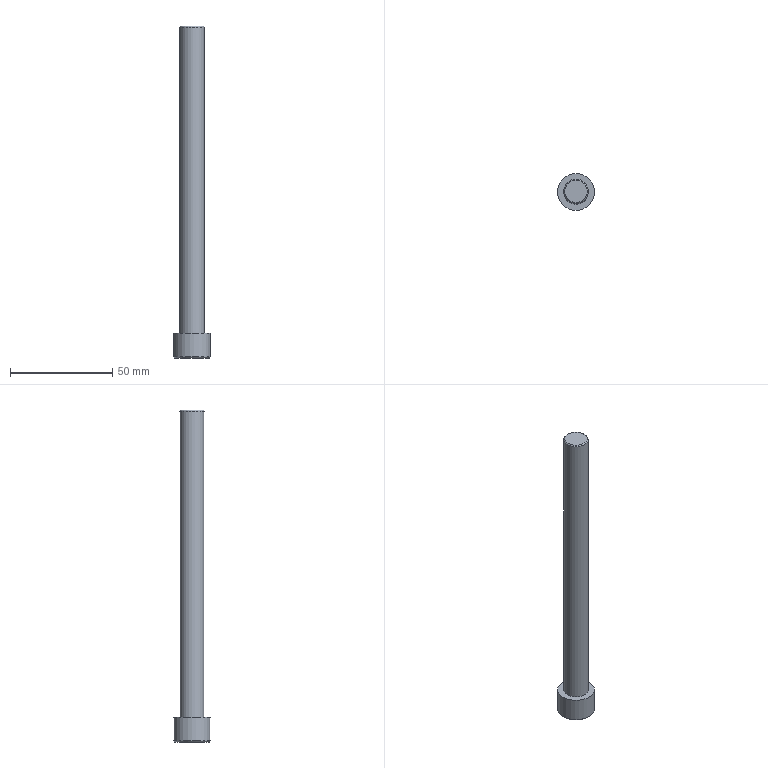Part | NX | features 19 2 | 1 solid | 20 faces | box 18 x 18 x 162 mm | volume 19452 mm3 | plane 15 | cone 3 | cylinder 2 | commonest cylinder face diameters 12 x1 18 x1
STEP:
#1=CARTESIAN_POINT('',(877.,320.774,-174.5));
#2=VERTEX_POINT('',#1);
#3=CARTESIAN_POINT('',(872.,317.887,-174.5));
#4=VERTEX_POINT('',#3);
#5=CARTESIAN_POINT('',(874.5,319.33,-174.5));
#6=DIRECTION('',(-0.866,-0.5,0.));
#7=VECTOR('',#6,1000.);
#8=LINE('',#5,#7);
#9=EDGE_CURVE('',#2,#4,#8,.T.);
#10=ORIENTED_EDGE('',*,*,#9,.F.);
#11=CARTESIAN_POINT('',(877.,315.,-174.5));
#12=DIRECTION('',(0.,0.,-1.));
#13=DIRECTION('',(-1.,0.,0.));
#14=AXIS2_PLACEMENT_3D('',#11,#12,#13);
#15=CIRCLE('',#14,5.774);
#16=EDGE_CURVE('',#4,#2,#15,.T.);
#17=ORIENTED_EDGE('',*,*,#16,.F.);
#18=EDGE_LOOP('',(#10,#17));
#19=FACE_BOUND('',#18,.T.);
#20=CARTESIAN_POINT('',(877.,315.,-174.5));
#21=DIRECTION('',(0.,0.,-1.));
#22=DIRECTION('',(1.,0.,0.));
#23=AXIS2_PLACEMENT_3D('',#20,#21,#22);
#24=PLANE('',#23);
#25=ADVANCED_FACE('',(#19),#24,.F.);
#26=CARTESIAN_POINT('',(872.,312.113,-174.5));
#27=VERTEX_POINT('',#26);
#28=CARTESIAN_POINT('',(872.,315.,-174.5));
#29=DIRECTION('',(0.,-1.,0.));
#30=VECTOR('',#29,1000.);
#31=LINE('',#28,#30);
#32=EDGE_CURVE('',#4,#27,#31,.T.);
#33=ORIENTED_EDGE('',*,*,#32,.F.);
#34=CARTESIAN_POINT('',(877.,315.,-174.5));
#35=DIRECTION('',(0.,0.,-1.));
#36=DIRECTION('',(-1.,0.,0.));
#37=AXIS2_PLACEMENT_3D('',#34,#35,#36);
#38=CIRCLE('',#37,5.774);
#39=EDGE_CURVE('',#27,#4,#38,.T.);
#40=ORIENTED_EDGE('',*,*,#39,.F.);
#41=EDGE_LOOP('',(#33,#40));
#42=FACE_BOUND('',#41,.T.);
#43=CARTESIAN_POINT('',(877.,315.,-174.5));
#44=DIRECTION('',(0.,0.,-1.));
#45=DIRECTION('',(1.,0.,0.));
#46=AXIS2_PLACEMENT_3D('',#43,#44,#45);
#47=PLANE('',#46);
#48=ADVANCED_FACE('',(#42),#47,.F.);
#49=CARTESIAN_POINT('',(877.,309.226,-174.5));
#50=VERTEX_POINT('',#49);
#51=CARTESIAN_POINT('',(874.5,310.67,-174.5));
#52=DIRECTION('',(0.866,-0.5,0.));
#53=VECTOR('',#52,1000.);
#54=LINE('',#51,#53);
#55=EDGE_CURVE('',#27,#50,#54,.T.);
#56=ORIENTED_EDGE('',*,*,#55,.F.);
#57=CARTESIAN_POINT('',(877.,315.,-174.5));
#58=DIRECTION('',(0.,0.,-1.));
#59=DIRECTION('',(-1.,0.,0.));
#60=AXIS2_PLACEMENT_3D('',#57,#58,#59);
#61=CIRCLE('',#60,5.774);
#62=EDGE_CURVE('',#50,#27,#61,.T.);
#63=ORIENTED_EDGE('',*,*,#62,.F.);
#64=EDGE_LOOP('',(#56,#63));
#65=FACE_BOUND('',#64,.T.);
#66=CARTESIAN_POINT('',(877.,315.,-174.5));
#67=DIRECTION('',(0.,0.,-1.));
#68=DIRECTION('',(1.,0.,0.));
#69=AXIS2_PLACEMENT_3D('',#66,#67,#68);
#70=PLANE('',#69);
#71=ADVANCED_FACE('',(#65),#70,.F.);
#72=CARTESIAN_POINT('',(882.,312.113,-174.5));
#73=VERTEX_POINT('',#72);
#74=CARTESIAN_POINT('',(879.5,310.67,-174.5));
#75=DIRECTION('',(0.866,0.5,0.));
#76=VECTOR('',#75,1000.);
#77=LINE('',#74,#76);
#78=EDGE_CURVE('',#50,#73,#77,.T.);
#79=ORIENTED_EDGE('',*,*,#78,.F.);
#80=CARTESIAN_POINT('',(877.,315.,-174.5));
#81=DIRECTION('',(0.,0.,-1.));
#82=DIRECTION('',(-1.,0.,0.));
#83=AXIS2_PLACEMENT_3D('',#80,#81,#82);
#84=CIRCLE('',#83,5.774);
#85=EDGE_CURVE('',#73,#50,#84,.T.);
#86=ORIENTED_EDGE('',*,*,#85,.F.);
#87=EDGE_LOOP('',(#79,#86));
#88=FACE_BOUND('',#87,.T.);
#89=CARTESIAN_POINT('',(877.,315.,-174.5));
#90=DIRECTION('',(0.,0.,-1.));
#91=DIRECTION('',(1.,0.,0.));
#92=AXIS2_PLACEMENT_3D('',#89,#90,#91);
#93=PLANE('',#92);
#94=ADVANCED_FACE('',(#88),#93,.F.);
#95=CARTESIAN_POINT('',(882.,317.887,-174.5));
#96=VERTEX_POINT('',#95);
#97=CARTESIAN_POINT('',(882.,315.,-174.5));
#98=DIRECTION('',(0.,1.,0.));
#99=VECTOR('',#98,1000.);
#100=LINE('',#97,#99);
#101=EDGE_CURVE('',#73,#96,#100,.T.);
#102=ORIENTED_EDGE('',*,*,#101,.F.);
#103=CARTESIAN_POINT('',(877.,315.,-174.5));
#104=DIRECTION('',(0.,0.,-1.));
#105=DIRECTION('',(-1.,0.,0.));
#106=AXIS2_PLACEMENT_3D('',#103,#104,#105);
#107=CIRCLE('',#106,5.774);
#108=EDGE_CURVE('',#96,#73,#107,.T.);
#109=ORIENTED_EDGE('',*,*,#108,.F.);
#110=EDGE_LOOP('',(#102,#109));
#111=FACE_BOUND('',#110,.T.);
#112=CARTESIAN_POINT('',(877.,315.,-174.5));
#113=DIRECTION('',(0.,0.,-1.));
#114=DIRECTION('',(1.,0.,0.));
#115=AXIS2_PLACEMENT_3D('',#112,#113,#114);
#116=PLANE('',#115);
#117=ADVANCED_FACE('',(#111),#116,.F.);
#118=CARTESIAN_POINT('',(879.5,319.33,-174.5));
#119=DIRECTION('',(-0.866,0.5,0.));
#120=VECTOR('',#119,1000.);
#121=LINE('',#118,#120);
#122=EDGE_CURVE('',#96,#2,#121,.T.);
#123=ORIENTED_EDGE('',*,*,#122,.F.);
#124=CARTESIAN_POINT('',(877.,315.,-174.5));
#125=DIRECTION('',(0.,0.,-1.));
#126=DIRECTION('',(-1.,0.,0.));
#127=AXIS2_PLACEMENT_3D('',#124,#125,#126);
#128=CIRCLE('',#127,5.774);
#129=EDGE_CURVE('',#2,#96,#128,.T.);
#130=ORIENTED_EDGE('',*,*,#129,.F.);
#131=EDGE_LOOP('',(#123,#130));
#132=FACE_BOUND('',#131,.T.);
#133=CARTESIAN_POINT('',(877.,315.,-174.5));
#134=DIRECTION('',(0.,0.,-1.));
#135=DIRECTION('',(1.,0.,0.));
#136=AXIS2_PLACEMENT_3D('',#133,#134,#135);
#137=PLANE('',#136);
#138=ADVANCED_FACE('',(#132),#137,.F.);
#139=ORIENTED_EDGE('',*,*,#39,.T.);
#140=ORIENTED_EDGE('',*,*,#16,.T.);
#141=ORIENTED_EDGE('',*,*,#129,.T.);
#142=ORIENTED_EDGE('',*,*,#108,.T.);
#143=ORIENTED_EDGE('',*,*,#85,.T.);
#144=ORIENTED_EDGE('',*,*,#62,.T.);
#145=EDGE_LOOP('',(#139,#140,#141,#142,#143,#144));
#146=FACE_BOUND('',#145,.T.);
#147=CARTESIAN_POINT('',(877.,315.,-173.5));
#148=VERTEX_POINT('',#147);
#149=VERTEX_LOOP('',#148);
#150=FACE_BOUND('',#149,.T.);
#151=CARTESIAN_POINT('',(877.,315.,-174.));
#152=DIRECTION('',(0.,0.,-1.));
#153=DIRECTION('',(-1.,0.,0.));
#154=AXIS2_PLACEMENT_3D('',#151,#152,#153);
#155=CONICAL_SURFACE('',#154,2.887,1.399);
#156=ADVANCED_FACE('',(#146,#150),#155,.F.);
#157=CARTESIAN_POINT('',(877.,320.774,-180.5));
#158=VERTEX_POINT('',#157);
#159=CARTESIAN_POINT('',(877.,320.774,-177.5));
#160=DIRECTION('',(0.,0.,-1.));
#161=VECTOR('',#160,1000.);
#162=LINE('',#159,#161);
#163=EDGE_CURVE('',#2,#158,#162,.T.);
#164=ORIENTED_EDGE('',*,*,#163,.F.);
#165=ORIENTED_EDGE('',*,*,#9,.T.);
#166=CARTESIAN_POINT('',(872.,317.887,-180.5));
#167=VERTEX_POINT('',#166);
#168=CARTESIAN_POINT('',(872.,317.887,-177.5));
#169=DIRECTION('',(0.,0.,-1.));
#170=VECTOR('',#169,1000.);
#171=LINE('',#168,#170);
#172=EDGE_CURVE('',#4,#167,#171,.T.);
#173=ORIENTED_EDGE('',*,*,#172,.T.);
#174=CARTESIAN_POINT('',(874.5,319.33,-180.5));
#175=DIRECTION('',(-0.866,-0.5,0.));
#176=VECTOR('',#175,1000.);
#177=LINE('',#174,#176);
#178=EDGE_CURVE('',#158,#167,#177,.T.);
#179=ORIENTED_EDGE('',*,*,#178,.F.);
#180=EDGE_LOOP('',(#164,#165,#173,#179));
#181=FACE_BOUND('',#180,.T.);
#182=CARTESIAN_POINT('',(874.5,319.33,-177.5));
#183=DIRECTION('',(0.5,-0.866,0.));
#184=DIRECTION('',(0.,0.,1.));
#185=AXIS2_PLACEMENT_3D('',#182,#183,#184);
#186=PLANE('',#185);
#187=ADVANCED_FACE('',(#181),#186,.T.);
#188=CARTESIAN_POINT('',(882.,317.887,-180.5));
#189=VERTEX_POINT('',#188);
#190=CARTESIAN_POINT('',(882.,317.887,-177.5));
#191=DIRECTION('',(0.,0.,-1.));
#192=VECTOR('',#191,1000.);
#193=LINE('',#190,#192);
#194=EDGE_CURVE('',#96,#189,#193,.T.);
#195=ORIENTED_EDGE('',*,*,#194,.F.);
#196=ORIENTED_EDGE('',*,*,#122,.T.);
#197=ORIENTED_EDGE('',*,*,#163,.T.);
#198=CARTESIAN_POINT('',(879.5,319.33,-180.5));
#199=DIRECTION('',(-0.866,0.5,0.));
#200=VECTOR('',#199,1000.);
#201=LINE('',#198,#200);
#202=EDGE_CURVE('',#189,#158,#201,.T.);
#203=ORIENTED_EDGE('',*,*,#202,.F.);
#204=EDGE_LOOP('',(#195,#196,#197,#203));
#205=FACE_BOUND('',#204,.T.);
#206=CARTESIAN_POINT('',(879.5,319.33,-177.5));
#207=DIRECTION('',(-0.5,-0.866,0.));
#208=DIRECTION('',(0.,0.,-1.));
#209=AXIS2_PLACEMENT_3D('',#206,#207,#208);
#210=PLANE('',#209);
#211=ADVANCED_FACE('',(#205),#210,.T.);
#212=CARTESIAN_POINT('',(882.,312.113,-180.5));
#213=VERTEX_POINT('',#212);
#214=CARTESIAN_POINT('',(882.,312.113,-177.5));
#215=DIRECTION('',(0.,0.,-1.));
#216=VECTOR('',#215,1000.);
#217=LINE('',#214,#216);
#218=EDGE_CURVE('',#73,#213,#217,.T.);
#219=ORIENTED_EDGE('',*,*,#218,.F.);
#220=ORIENTED_EDGE('',*,*,#101,.T.);
#221=ORIENTED_EDGE('',*,*,#194,.T.);
#222=CARTESIAN_POINT('',(882.,315.,-180.5));
#223=DIRECTION('',(0.,1.,0.));
#224=VECTOR('',#223,1000.);
#225=LINE('',#222,#224);
#226=EDGE_CURVE('',#213,#189,#225,.T.);
#227=ORIENTED_EDGE('',*,*,#226,.F.);
#228=EDGE_LOOP('',(#219,#220,#221,#227));
#229=FACE_BOUND('',#228,.T.);
#230=CARTESIAN_POINT('',(882.,315.,-177.5));
#231=DIRECTION('',(-1.,0.,0.));
#232=DIRECTION('',(0.,0.,-1.));
#233=AXIS2_PLACEMENT_3D('',#230,#231,#232);
#234=PLANE('',#233);
#235=ADVANCED_FACE('',(#229),#234,.T.);
#236=CARTESIAN_POINT('',(877.,309.226,-180.5));
#237=VERTEX_POINT('',#236);
#238=CARTESIAN_POINT('',(877.,309.226,-177.5));
#239=DIRECTION('',(0.,0.,-1.));
#240=VECTOR('',#239,1000.);
#241=LINE('',#238,#240);
#242=EDGE_CURVE('',#50,#237,#241,.T.);
#243=ORIENTED_EDGE('',*,*,#242,.F.);
#244=ORIENTED_EDGE('',*,*,#78,.T.);
#245=ORIENTED_EDGE('',*,*,#218,.T.);
#246=CARTESIAN_POINT('',(879.5,310.67,-180.5));
#247=DIRECTION('',(0.866,0.5,0.));
#248=VECTOR('',#247,1000.);
#249=LINE('',#246,#248);
#250=EDGE_CURVE('',#237,#213,#249,.T.);
#251=ORIENTED_EDGE('',*,*,#250,.F.);
#252=EDGE_LOOP('',(#243,#244,#245,#251));
#253=FACE_BOUND('',#252,.T.);
#254=CARTESIAN_POINT('',(879.5,310.67,-177.5));
#255=DIRECTION('',(-0.5,0.866,0.));
#256=DIRECTION('',(0.,0.,-1.));
#257=AXIS2_PLACEMENT_3D('',#254,#255,#256);
#258=PLANE('',#257);
#259=ADVANCED_FACE('',(#253),#258,.T.);
#260=CARTESIAN_POINT('',(872.,312.113,-180.5));
#261=VERTEX_POINT('',#260);
#262=CARTESIAN_POINT('',(872.,312.113,-177.5));
#263=DIRECTION('',(0.,0.,-1.));
#264=VECTOR('',#263,1000.);
#265=LINE('',#262,#264);
#266=EDGE_CURVE('',#27,#261,#265,.T.);
#267=ORIENTED_EDGE('',*,*,#266,.F.);
#268=ORIENTED_EDGE('',*,*,#55,.T.);
#269=ORIENTED_EDGE('',*,*,#242,.T.);
#270=CARTESIAN_POINT('',(874.5,310.67,-180.5));
#271=DIRECTION('',(0.866,-0.5,0.));
#272=VECTOR('',#271,1000.);
#273=LINE('',#270,#272);
#274=EDGE_CURVE('',#261,#237,#273,.T.);
#275=ORIENTED_EDGE('',*,*,#274,.F.);
#276=EDGE_LOOP('',(#267,#268,#269,#275));
#277=FACE_BOUND('',#276,.T.);
#278=CARTESIAN_POINT('',(874.5,310.67,-177.5));
#279=DIRECTION('',(0.5,0.866,0.));
#280=DIRECTION('',(0.,0.,1.));
#281=AXIS2_PLACEMENT_3D('',#278,#279,#280);
#282=PLANE('',#281);
#283=ADVANCED_FACE('',(#277),#282,.T.);
#284=ORIENTED_EDGE('',*,*,#172,.F.);
#285=ORIENTED_EDGE('',*,*,#32,.T.);
#286=ORIENTED_EDGE('',*,*,#266,.T.);
#287=CARTESIAN_POINT('',(872.,315.,-180.5));
#288=DIRECTION('',(0.,-1.,0.));
#289=VECTOR('',#288,1000.);
#290=LINE('',#287,#289);
#291=EDGE_CURVE('',#167,#261,#290,.T.);
#292=ORIENTED_EDGE('',*,*,#291,.F.);
#293=EDGE_LOOP('',(#284,#285,#286,#292));
#294=FACE_BOUND('',#293,.T.);
#295=CARTESIAN_POINT('',(872.,315.,-177.5));
#296=DIRECTION('',(1.,0.,0.));
#297=DIRECTION('',(0.,0.,1.));
#298=AXIS2_PLACEMENT_3D('',#295,#296,#297);
#299=PLANE('',#298);
#300=ADVANCED_FACE('',(#294),#299,.T.);
#301=CARTESIAN_POINT('',(871.,315.,-19.));
#302=VERTEX_POINT('',#301);
#303=CARTESIAN_POINT('',(877.,315.,-19.));
#304=DIRECTION('',(0.,0.,1.));
#305=DIRECTION('',(1.,0.,0.));
#306=AXIS2_PLACEMENT_3D('',#303,#304,#305);
#307=CIRCLE('',#306,6.);
#308=EDGE_CURVE('',#302,#302,#307,.T.);
#309=ORIENTED_EDGE('',*,*,#308,.T.);
#310=EDGE_LOOP('',(#309));
#311=FACE_BOUND('',#310,.T.);
#312=CARTESIAN_POINT('',(871.5,315.,-18.5));
#313=VERTEX_POINT('',#312);
#314=CARTESIAN_POINT('',(877.,315.,-18.5));
#315=DIRECTION('',(0.,0.,-1.));
#316=DIRECTION('',(1.,0.,0.));
#317=AXIS2_PLACEMENT_3D('',#314,#315,#316);
#318=CIRCLE('',#317,5.5);
#319=EDGE_CURVE('',#313,#313,#318,.T.);
#320=ORIENTED_EDGE('',*,*,#319,.T.);
#321=EDGE_LOOP('',(#320));
#322=FACE_BOUND('',#321,.T.);
#323=CARTESIAN_POINT('',(877.,315.,-18.5));
#324=DIRECTION('',(0.,0.,-1.));
#325=DIRECTION('',(1.,0.,0.));
#326=AXIS2_PLACEMENT_3D('',#323,#324,#325);
#327=CONICAL_SURFACE('',#326,5.5,0.7854);
#328=ADVANCED_FACE('',(#311,#322),#327,.T.);
#329=CARTESIAN_POINT('',(871.,315.,-168.5));
#330=VERTEX_POINT('',#329);
#331=CARTESIAN_POINT('',(877.,315.,-168.5));
#332=DIRECTION('',(0.,0.,-1.));
#333=DIRECTION('',(-1.,0.,0.));
#334=AXIS2_PLACEMENT_3D('',#331,#332,#333);
#335=CIRCLE('',#334,6.);
#336=EDGE_CURVE('',#330,#330,#335,.T.);
#337=ORIENTED_EDGE('',*,*,#336,.F.);
#338=EDGE_LOOP('',(#337));
#339=FACE_BOUND('',#338,.T.);
#340=ORIENTED_EDGE('',*,*,#308,.F.);
#341=EDGE_LOOP('',(#340));
#342=FACE_BOUND('',#341,.T.);
#343=CARTESIAN_POINT('',(877.,315.,-83.5));
#344=DIRECTION('',(0.,0.,1.));
#345=DIRECTION('',(-1.,0.,0.));
#346=AXIS2_PLACEMENT_3D('',#343,#344,#345);
#347=CYLINDRICAL_SURFACE('',#346,6.);
#348=ADVANCED_FACE('',(#339,#342),#347,.T.);
#349=ORIENTED_EDGE('',*,*,#319,.F.);
#350=EDGE_LOOP('',(#349));
#351=FACE_BOUND('',#350,.T.);
#352=CARTESIAN_POINT('',(877.,315.,-18.5));
#353=DIRECTION('',(0.,0.,1.));
#354=DIRECTION('',(-1.,0.,0.));
#355=AXIS2_PLACEMENT_3D('',#352,#353,#354);
#356=PLANE('',#355);
#357=ADVANCED_FACE('',(#351),#356,.T.);
#358=CARTESIAN_POINT('',(868.,315.,-180.));
#359=VERTEX_POINT('',#358);
#360=CARTESIAN_POINT('',(877.,315.,-180.));
#361=DIRECTION('',(0.,0.,-1.));
#362=DIRECTION('',(1.,0.,0.));
#363=AXIS2_PLACEMENT_3D('',#360,#361,#362);
#364=CIRCLE('',#363,9.);
#365=EDGE_CURVE('',#359,#359,#364,.T.);
#366=ORIENTED_EDGE('',*,*,#365,.T.);
#367=EDGE_LOOP('',(#366));
#368=FACE_BOUND('',#367,.T.);
#369=CARTESIAN_POINT('',(868.5,315.,-180.5));
#370=VERTEX_POINT('',#369);
#371=CARTESIAN_POINT('',(877.,315.,-180.5));
#372=DIRECTION('',(0.,0.,1.));
#373=DIRECTION('',(1.,0.,0.));
#374=AXIS2_PLACEMENT_3D('',#371,#372,#373);
#375=CIRCLE('',#374,8.5);
#376=EDGE_CURVE('',#370,#370,#375,.T.);
#377=ORIENTED_EDGE('',*,*,#376,.T.);
#378=EDGE_LOOP('',(#377));
#379=FACE_BOUND('',#378,.T.);
#380=CARTESIAN_POINT('',(877.,315.,-180.5));
#381=DIRECTION('',(0.,0.,1.));
#382=DIRECTION('',(1.,0.,0.));
#383=AXIS2_PLACEMENT_3D('',#380,#381,#382);
#384=CONICAL_SURFACE('',#383,8.5,0.7854);
#385=ADVANCED_FACE('',(#368,#379),#384,.T.);
#386=CARTESIAN_POINT('',(868.,315.,-168.5));
#387=VERTEX_POINT('',#386);
#388=CARTESIAN_POINT('',(877.,315.,-168.5));
#389=DIRECTION('',(0.,0.,1.));
#390=DIRECTION('',(-1.,0.,0.));
#391=AXIS2_PLACEMENT_3D('',#388,#389,#390);
#392=CIRCLE('',#391,9.);
#393=EDGE_CURVE('',#387,#387,#392,.T.);
#394=ORIENTED_EDGE('',*,*,#393,.F.);
#395=EDGE_LOOP('',(#394));
#396=FACE_BOUND('',#395,.T.);
#397=ORIENTED_EDGE('',*,*,#365,.F.);
#398=EDGE_LOOP('',(#397));
#399=FACE_BOUND('',#398,.T.);
#400=CARTESIAN_POINT('',(877.,315.,-174.5));
#401=DIRECTION('',(0.,0.,1.));
#402=DIRECTION('',(-1.,0.,0.));
#403=AXIS2_PLACEMENT_3D('',#400,#401,#402);
#404=CYLINDRICAL_SURFACE('',#403,9.);
#405=ADVANCED_FACE('',(#396,#399),#404,.T.);
#406=ORIENTED_EDGE('',*,*,#178,.T.);
#407=ORIENTED_EDGE('',*,*,#291,.T.);
#408=ORIENTED_EDGE('',*,*,#274,.T.);
#409=ORIENTED_EDGE('',*,*,#250,.T.);
#410=ORIENTED_EDGE('',*,*,#226,.T.);
#411=ORIENTED_EDGE('',*,*,#202,.T.);
#412=EDGE_LOOP('',(#406,#407,#408,#409,#410,#411));
#413=FACE_BOUND('',#412,.T.);
#414=ORIENTED_EDGE('',*,*,#376,.F.);
#415=EDGE_LOOP('',(#414));
#416=FACE_BOUND('',#415,.T.);
#417=CARTESIAN_POINT('',(877.,315.,-180.5));
#418=DIRECTION('',(0.,0.,-1.));
#419=DIRECTION('',(1.,0.,0.));
#420=AXIS2_PLACEMENT_3D('',#417,#418,#419);
#421=PLANE('',#420);
#422=ADVANCED_FACE('',(#413,#416),#421,.T.);
#423=ORIENTED_EDGE('',*,*,#336,.T.);
#424=EDGE_LOOP('',(#423));
#425=FACE_BOUND('',#424,.T.);
#426=ORIENTED_EDGE('',*,*,#393,.T.);
#427=EDGE_LOOP('',(#426));
#428=FACE_BOUND('',#427,.T.);
#429=CARTESIAN_POINT('',(877.,315.,-168.5));
#430=DIRECTION('',(0.,0.,1.));
#431=DIRECTION('',(-1.,0.,0.));
#432=AXIS2_PLACEMENT_3D('',#429,#430,#431);
#433=PLANE('',#432);
#434=ADVANCED_FACE('',(#425,#428),#433,.T.);
#435=CLOSED_SHELL('',(#25,#48,#71,#94,#117,#138,#156,#187,#211,#235,#259,#283,#300,#328,#348,#357,#385,#405,#422,#434));
#436=MANIFOLD_SOLID_BREP('',#435);
#437=(LENGTH_UNIT()NAMED_UNIT(*)SI_UNIT(.MILLI.,.METRE.));
#438=UNCERTAINTY_MEASURE_WITH_UNIT(LENGTH_MEASURE(0.00001),#437,'','');
#439=(NAMED_UNIT(*)PLANE_ANGLE_UNIT()SI_UNIT($,.RADIAN.));
#440=(NAMED_UNIT(*)SI_UNIT($,.STERADIAN.)SOLID_ANGLE_UNIT());
#441=(GEOMETRIC_REPRESENTATION_CONTEXT(3)GLOBAL_UNCERTAINTY_ASSIGNED_CONTEXT((#438))GLOBAL_UNIT_ASSIGNED_CONTEXT((#437,#439,#440))REPRESENTATION_CONTEXT('',''));
#442=ADVANCED_BREP_SHAPE_REPRESENTATION('',(#436),#441);